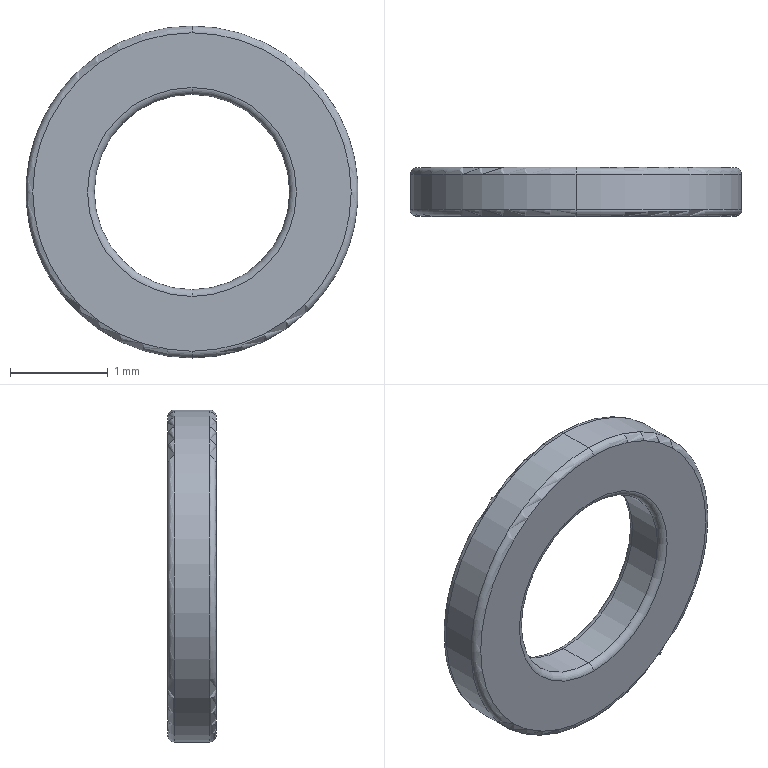Part | SolidWorks | features Extrusion 1, Fillet 1 | 1 solid | 14 faces | box 3.4 x 0.5 x 3.4 mm | volume 2.933 mm3 | torus 8 | cylinder 4 | plane 2 | commonest cylinder face diameters 2 x2 3.4 x2
STEP:
#1=CARTESIAN_POINT('',(0.,0.43,-1.7));
#2=VERTEX_POINT('',#1);
#3=CARTESIAN_POINT('',(0.,0.43,1.7));
#4=VERTEX_POINT('',#3);
#5=CARTESIAN_POINT('',(0.,0.43,0.));
#6=DIRECTION('',(0.,-1.,0.));
#7=DIRECTION('',(0.,0.,1.));
#8=AXIS2_PLACEMENT_3D('',#5,#6,#7);
#9=CIRCLE('',#8,1.7);
#10=EDGE_CURVE('',#2,#4,#9,.T.);
#11=ORIENTED_EDGE('',*,*,#10,.F.);
#12=CARTESIAN_POINT('',(0.,0.5,-1.63));
#13=VERTEX_POINT('',#12);
#14=CARTESIAN_POINT('',(0.,0.43,-1.63));
#15=DIRECTION('',(1.,0.,0.));
#16=DIRECTION('',(0.,0.,-1.));
#17=AXIS2_PLACEMENT_3D('',#14,#15,#16);
#18=CIRCLE('',#17,0.07);
#19=EDGE_CURVE('',#2,#13,#18,.T.);
#20=ORIENTED_EDGE('',*,*,#19,.T.);
#21=CARTESIAN_POINT('',(0.,0.5,1.63));
#22=VERTEX_POINT('',#21);
#23=CARTESIAN_POINT('',(0.,0.5,0.));
#24=DIRECTION('',(0.,1.,0.));
#25=DIRECTION('',(0.,0.,1.));
#26=AXIS2_PLACEMENT_3D('',#23,#24,#25);
#27=CIRCLE('',#26,1.63);
#28=EDGE_CURVE('',#22,#13,#27,.T.);
#29=ORIENTED_EDGE('',*,*,#28,.F.);
#30=CARTESIAN_POINT('',(0.,0.43,1.63));
#31=DIRECTION('',(-1.,0.,0.));
#32=DIRECTION('',(0.,0.,1.));
#33=AXIS2_PLACEMENT_3D('',#30,#31,#32);
#34=CIRCLE('',#33,0.07);
#35=EDGE_CURVE('',#4,#22,#34,.T.);
#36=ORIENTED_EDGE('',*,*,#35,.F.);
#37=EDGE_LOOP('',(#11,#20,#29,#36));
#38=FACE_OUTER_BOUND('',#37,.T.);
#39=CARTESIAN_POINT('',(0.,0.43,0.));
#40=DIRECTION('',(0.,1.,0.));
#41=DIRECTION('',(0.,0.,1.));
#42=AXIS2_PLACEMENT_3D('',#39,#40,#41);
#43=TOROIDAL_SURFACE('',#42,1.63,0.07);
#44=ADVANCED_FACE('',(#38),#43,.T.);
#45=CARTESIAN_POINT('',(0.,0.,-1.63));
#46=VERTEX_POINT('',#45);
#47=CARTESIAN_POINT('',(0.,0.,1.63));
#48=VERTEX_POINT('',#47);
#49=CARTESIAN_POINT('',(0.,0.,0.));
#50=DIRECTION('',(0.,-1.,0.));
#51=DIRECTION('',(0.,0.,1.));
#52=AXIS2_PLACEMENT_3D('',#49,#50,#51);
#53=CIRCLE('',#52,1.63);
#54=EDGE_CURVE('',#46,#48,#53,.T.);
#55=ORIENTED_EDGE('',*,*,#54,.F.);
#56=CARTESIAN_POINT('',(0.,0.07,-1.7));
#57=VERTEX_POINT('',#56);
#58=CARTESIAN_POINT('',(0.,0.07,-1.63));
#59=DIRECTION('',(1.,0.,0.));
#60=DIRECTION('',(0.,0.,-1.));
#61=AXIS2_PLACEMENT_3D('',#58,#59,#60);
#62=CIRCLE('',#61,0.07);
#63=EDGE_CURVE('',#46,#57,#62,.T.);
#64=ORIENTED_EDGE('',*,*,#63,.T.);
#65=CARTESIAN_POINT('',(0.,0.07,1.7));
#66=VERTEX_POINT('',#65);
#67=CARTESIAN_POINT('',(0.,0.07,0.));
#68=DIRECTION('',(0.,1.,0.));
#69=DIRECTION('',(0.,0.,1.));
#70=AXIS2_PLACEMENT_3D('',#67,#68,#69);
#71=CIRCLE('',#70,1.7);
#72=EDGE_CURVE('',#66,#57,#71,.T.);
#73=ORIENTED_EDGE('',*,*,#72,.F.);
#74=CARTESIAN_POINT('',(0.,0.07,1.63));
#75=DIRECTION('',(-1.,0.,0.));
#76=DIRECTION('',(0.,0.,1.));
#77=AXIS2_PLACEMENT_3D('',#74,#75,#76);
#78=CIRCLE('',#77,0.07);
#79=EDGE_CURVE('',#48,#66,#78,.T.);
#80=ORIENTED_EDGE('',*,*,#79,.F.);
#81=EDGE_LOOP('',(#55,#64,#73,#80));
#82=FACE_OUTER_BOUND('',#81,.T.);
#83=CARTESIAN_POINT('',(0.,0.07,0.));
#84=DIRECTION('',(0.,1.,0.));
#85=DIRECTION('',(0.,0.,1.));
#86=AXIS2_PLACEMENT_3D('',#83,#84,#85);
#87=TOROIDAL_SURFACE('',#86,1.63,0.07);
#88=ADVANCED_FACE('',(#82),#87,.T.);
#89=CARTESIAN_POINT('',(0.,0.5,-1.07));
#90=VERTEX_POINT('',#89);
#91=CARTESIAN_POINT('',(0.,0.5,1.07));
#92=VERTEX_POINT('',#91);
#93=CARTESIAN_POINT('',(0.,0.5,0.));
#94=DIRECTION('',(0.,-1.,0.));
#95=DIRECTION('',(0.,0.,1.));
#96=AXIS2_PLACEMENT_3D('',#93,#94,#95);
#97=CIRCLE('',#96,1.07);
#98=EDGE_CURVE('',#90,#92,#97,.T.);
#99=ORIENTED_EDGE('',*,*,#98,.F.);
#100=CARTESIAN_POINT('',(0.,0.43,-1.));
#101=VERTEX_POINT('',#100);
#102=CARTESIAN_POINT('',(0.,0.43,-1.07));
#103=DIRECTION('',(1.,0.,0.));
#104=DIRECTION('',(0.,0.,-1.));
#105=AXIS2_PLACEMENT_3D('',#102,#103,#104);
#106=CIRCLE('',#105,0.07);
#107=EDGE_CURVE('',#90,#101,#106,.T.);
#108=ORIENTED_EDGE('',*,*,#107,.T.);
#109=CARTESIAN_POINT('',(0.,0.43,1.));
#110=VERTEX_POINT('',#109);
#111=CARTESIAN_POINT('',(0.,0.43,0.));
#112=DIRECTION('',(0.,1.,0.));
#113=DIRECTION('',(0.,0.,1.));
#114=AXIS2_PLACEMENT_3D('',#111,#112,#113);
#115=CIRCLE('',#114,1.);
#116=EDGE_CURVE('',#110,#101,#115,.T.);
#117=ORIENTED_EDGE('',*,*,#116,.F.);
#118=CARTESIAN_POINT('',(0.,0.43,1.07));
#119=DIRECTION('',(-1.,0.,0.));
#120=DIRECTION('',(0.,0.,1.));
#121=AXIS2_PLACEMENT_3D('',#118,#119,#120);
#122=CIRCLE('',#121,0.07);
#123=EDGE_CURVE('',#92,#110,#122,.T.);
#124=ORIENTED_EDGE('',*,*,#123,.F.);
#125=EDGE_LOOP('',(#99,#108,#117,#124));
#126=FACE_OUTER_BOUND('',#125,.T.);
#127=CARTESIAN_POINT('',(0.,0.43,0.));
#128=DIRECTION('',(0.,1.,0.));
#129=DIRECTION('',(0.,0.,1.));
#130=AXIS2_PLACEMENT_3D('',#127,#128,#129);
#131=TOROIDAL_SURFACE('',#130,1.07,0.07);
#132=ADVANCED_FACE('',(#126),#131,.T.);
#133=CARTESIAN_POINT('',(0.,0.07,-1.));
#134=VERTEX_POINT('',#133);
#135=CARTESIAN_POINT('',(0.,0.07,1.));
#136=VERTEX_POINT('',#135);
#137=CARTESIAN_POINT('',(0.,0.07,0.));
#138=DIRECTION('',(0.,-1.,0.));
#139=DIRECTION('',(0.,0.,1.));
#140=AXIS2_PLACEMENT_3D('',#137,#138,#139);
#141=CIRCLE('',#140,1.);
#142=EDGE_CURVE('',#134,#136,#141,.T.);
#143=ORIENTED_EDGE('',*,*,#142,.F.);
#144=CARTESIAN_POINT('',(0.,0.,-1.07));
#145=VERTEX_POINT('',#144);
#146=CARTESIAN_POINT('',(0.,0.07,-1.07));
#147=DIRECTION('',(1.,0.,0.));
#148=DIRECTION('',(0.,0.,-1.));
#149=AXIS2_PLACEMENT_3D('',#146,#147,#148);
#150=CIRCLE('',#149,0.07);
#151=EDGE_CURVE('',#134,#145,#150,.T.);
#152=ORIENTED_EDGE('',*,*,#151,.T.);
#153=CARTESIAN_POINT('',(0.,0.,1.07));
#154=VERTEX_POINT('',#153);
#155=CARTESIAN_POINT('',(0.,0.,0.));
#156=DIRECTION('',(0.,1.,0.));
#157=DIRECTION('',(0.,0.,1.));
#158=AXIS2_PLACEMENT_3D('',#155,#156,#157);
#159=CIRCLE('',#158,1.07);
#160=EDGE_CURVE('',#154,#145,#159,.T.);
#161=ORIENTED_EDGE('',*,*,#160,.F.);
#162=CARTESIAN_POINT('',(0.,0.07,1.07));
#163=DIRECTION('',(-1.,0.,0.));
#164=DIRECTION('',(0.,0.,1.));
#165=AXIS2_PLACEMENT_3D('',#162,#163,#164);
#166=CIRCLE('',#165,0.07);
#167=EDGE_CURVE('',#136,#154,#166,.T.);
#168=ORIENTED_EDGE('',*,*,#167,.F.);
#169=EDGE_LOOP('',(#143,#152,#161,#168));
#170=FACE_OUTER_BOUND('',#169,.T.);
#171=CARTESIAN_POINT('',(0.,0.07,0.));
#172=DIRECTION('',(0.,1.,0.));
#173=DIRECTION('',(0.,0.,1.));
#174=AXIS2_PLACEMENT_3D('',#171,#172,#173);
#175=TOROIDAL_SURFACE('',#174,1.07,0.07);
#176=ADVANCED_FACE('',(#170),#175,.T.);
#177=CARTESIAN_POINT('',(0.,0.43,0.));
#178=DIRECTION('',(0.,1.,0.));
#179=DIRECTION('',(0.,0.,1.));
#180=AXIS2_PLACEMENT_3D('',#177,#178,#179);
#181=CIRCLE('',#180,1.);
#182=EDGE_CURVE('',#101,#110,#181,.T.);
#183=ORIENTED_EDGE('',*,*,#182,.T.);
#184=CARTESIAN_POINT('',(0.,0.5,1.));
#185=DIRECTION('',(0.,-1.,0.));
#186=VECTOR('',#185,1000.);
#187=LINE('',#184,#186);
#188=EDGE_CURVE('',#110,#136,#187,.T.);
#189=ORIENTED_EDGE('',*,*,#188,.T.);
#190=CARTESIAN_POINT('',(0.,0.07,0.));
#191=DIRECTION('',(0.,-1.,0.));
#192=DIRECTION('',(0.,0.,1.));
#193=AXIS2_PLACEMENT_3D('',#190,#191,#192);
#194=CIRCLE('',#193,1.);
#195=EDGE_CURVE('',#136,#134,#194,.T.);
#196=ORIENTED_EDGE('',*,*,#195,.T.);
#197=CARTESIAN_POINT('',(0.,0.5,-1.));
#198=DIRECTION('',(0.,-1.,0.));
#199=VECTOR('',#198,1000.);
#200=LINE('',#197,#199);
#201=EDGE_CURVE('',#101,#134,#200,.T.);
#202=ORIENTED_EDGE('',*,*,#201,.F.);
#203=EDGE_LOOP('',(#183,#189,#196,#202));
#204=FACE_OUTER_BOUND('',#203,.T.);
#205=CARTESIAN_POINT('',(0.,0.5,0.));
#206=DIRECTION('',(0.,-1.,0.));
#207=DIRECTION('',(0.,0.,-1.));
#208=AXIS2_PLACEMENT_3D('',#205,#206,#207);
#209=CYLINDRICAL_SURFACE('',#208,1.);
#210=ADVANCED_FACE('',(#204),#209,.F.);
#211=ORIENTED_EDGE('',*,*,#10,.T.);
#212=CARTESIAN_POINT('',(0.,0.5,1.7));
#213=DIRECTION('',(0.,-1.,0.));
#214=VECTOR('',#213,1000.);
#215=LINE('',#212,#214);
#216=EDGE_CURVE('',#4,#66,#215,.T.);
#217=ORIENTED_EDGE('',*,*,#216,.T.);
#218=ORIENTED_EDGE('',*,*,#72,.T.);
#219=CARTESIAN_POINT('',(0.,0.5,-1.7));
#220=DIRECTION('',(0.,-1.,0.));
#221=VECTOR('',#220,1000.);
#222=LINE('',#219,#221);
#223=EDGE_CURVE('',#2,#57,#222,.T.);
#224=ORIENTED_EDGE('',*,*,#223,.F.);
#225=EDGE_LOOP('',(#211,#217,#218,#224));
#226=FACE_OUTER_BOUND('',#225,.T.);
#227=CARTESIAN_POINT('',(0.,0.5,0.));
#228=DIRECTION('',(0.,-1.,0.));
#229=DIRECTION('',(0.,0.,-1.));
#230=AXIS2_PLACEMENT_3D('',#227,#228,#229);
#231=CYLINDRICAL_SURFACE('',#230,1.7);
#232=ADVANCED_FACE('',(#226),#231,.T.);
#233=CARTESIAN_POINT('',(0.,0.5,0.));
#234=DIRECTION('',(0.,-1.,0.));
#235=DIRECTION('',(0.,0.,1.));
#236=AXIS2_PLACEMENT_3D('',#233,#234,#235);
#237=CIRCLE('',#236,1.07);
#238=EDGE_CURVE('',#92,#90,#237,.T.);
#239=ORIENTED_EDGE('',*,*,#238,.T.);
#240=ORIENTED_EDGE('',*,*,#98,.T.);
#241=EDGE_LOOP('',(#239,#240));
#242=FACE_BOUND('',#241,.T.);
#243=ORIENTED_EDGE('',*,*,#28,.T.);
#244=CARTESIAN_POINT('',(0.,0.5,0.));
#245=DIRECTION('',(0.,1.,0.));
#246=DIRECTION('',(0.,0.,1.));
#247=AXIS2_PLACEMENT_3D('',#244,#245,#246);
#248=CIRCLE('',#247,1.63);
#249=EDGE_CURVE('',#13,#22,#248,.T.);
#250=ORIENTED_EDGE('',*,*,#249,.T.);
#251=EDGE_LOOP('',(#243,#250));
#252=FACE_OUTER_BOUND('',#251,.T.);
#253=CARTESIAN_POINT('',(0.,0.5,0.));
#254=DIRECTION('',(0.,1.,0.));
#255=DIRECTION('',(0.,0.,1.));
#256=AXIS2_PLACEMENT_3D('',#253,#254,#255);
#257=PLANE('',#256);
#258=ADVANCED_FACE('',(#242,#252),#257,.T.);
#259=ORIENTED_EDGE('',*,*,#160,.T.);
#260=CARTESIAN_POINT('',(0.,0.,0.));
#261=DIRECTION('',(0.,1.,0.));
#262=DIRECTION('',(0.,0.,1.));
#263=AXIS2_PLACEMENT_3D('',#260,#261,#262);
#264=CIRCLE('',#263,1.07);
#265=EDGE_CURVE('',#145,#154,#264,.T.);
#266=ORIENTED_EDGE('',*,*,#265,.T.);
#267=EDGE_LOOP('',(#259,#266));
#268=FACE_BOUND('',#267,.T.);
#269=CARTESIAN_POINT('',(0.,0.,0.));
#270=DIRECTION('',(0.,-1.,0.));
#271=DIRECTION('',(0.,0.,1.));
#272=AXIS2_PLACEMENT_3D('',#269,#270,#271);
#273=CIRCLE('',#272,1.63);
#274=EDGE_CURVE('',#48,#46,#273,.T.);
#275=ORIENTED_EDGE('',*,*,#274,.T.);
#276=ORIENTED_EDGE('',*,*,#54,.T.);
#277=EDGE_LOOP('',(#275,#276));
#278=FACE_OUTER_BOUND('',#277,.T.);
#279=CARTESIAN_POINT('',(0.,0.,0.));
#280=DIRECTION('',(0.,1.,0.));
#281=DIRECTION('',(0.,0.,1.));
#282=AXIS2_PLACEMENT_3D('',#279,#280,#281);
#283=PLANE('',#282);
#284=ADVANCED_FACE('',(#268,#278),#283,.F.);
#285=ORIENTED_EDGE('',*,*,#216,.F.);
#286=CARTESIAN_POINT('',(0.,0.43,0.));
#287=DIRECTION('',(0.,-1.,0.));
#288=DIRECTION('',(0.,0.,1.));
#289=AXIS2_PLACEMENT_3D('',#286,#287,#288);
#290=CIRCLE('',#289,1.7);
#291=EDGE_CURVE('',#4,#2,#290,.T.);
#292=ORIENTED_EDGE('',*,*,#291,.T.);
#293=ORIENTED_EDGE('',*,*,#223,.T.);
#294=CARTESIAN_POINT('',(0.,0.07,0.));
#295=DIRECTION('',(0.,1.,0.));
#296=DIRECTION('',(0.,0.,1.));
#297=AXIS2_PLACEMENT_3D('',#294,#295,#296);
#298=CIRCLE('',#297,1.7);
#299=EDGE_CURVE('',#57,#66,#298,.T.);
#300=ORIENTED_EDGE('',*,*,#299,.T.);
#301=EDGE_LOOP('',(#285,#292,#293,#300));
#302=FACE_OUTER_BOUND('',#301,.T.);
#303=CARTESIAN_POINT('',(0.,0.5,0.));
#304=DIRECTION('',(0.,-1.,0.));
#305=DIRECTION('',(0.,0.,-1.));
#306=AXIS2_PLACEMENT_3D('',#303,#304,#305);
#307=CYLINDRICAL_SURFACE('',#306,1.7);
#308=ADVANCED_FACE('',(#302),#307,.T.);
#309=ORIENTED_EDGE('',*,*,#188,.F.);
#310=ORIENTED_EDGE('',*,*,#116,.T.);
#311=ORIENTED_EDGE('',*,*,#201,.T.);
#312=ORIENTED_EDGE('',*,*,#142,.T.);
#313=EDGE_LOOP('',(#309,#310,#311,#312));
#314=FACE_OUTER_BOUND('',#313,.T.);
#315=CARTESIAN_POINT('',(0.,0.5,0.));
#316=DIRECTION('',(0.,-1.,0.));
#317=DIRECTION('',(0.,0.,-1.));
#318=AXIS2_PLACEMENT_3D('',#315,#316,#317);
#319=CYLINDRICAL_SURFACE('',#318,1.);
#320=ADVANCED_FACE('',(#314),#319,.F.);
#321=ORIENTED_EDGE('',*,*,#151,.F.);
#322=ORIENTED_EDGE('',*,*,#195,.F.);
#323=ORIENTED_EDGE('',*,*,#167,.T.);
#324=ORIENTED_EDGE('',*,*,#265,.F.);
#325=EDGE_LOOP('',(#321,#322,#323,#324));
#326=FACE_OUTER_BOUND('',#325,.T.);
#327=CARTESIAN_POINT('',(0.,0.07,0.));
#328=DIRECTION('',(0.,1.,0.));
#329=DIRECTION('',(0.,0.,1.));
#330=AXIS2_PLACEMENT_3D('',#327,#328,#329);
#331=TOROIDAL_SURFACE('',#330,1.07,0.07);
#332=ADVANCED_FACE('',(#326),#331,.T.);
#333=ORIENTED_EDGE('',*,*,#107,.F.);
#334=ORIENTED_EDGE('',*,*,#238,.F.);
#335=ORIENTED_EDGE('',*,*,#123,.T.);
#336=ORIENTED_EDGE('',*,*,#182,.F.);
#337=EDGE_LOOP('',(#333,#334,#335,#336));
#338=FACE_OUTER_BOUND('',#337,.T.);
#339=CARTESIAN_POINT('',(0.,0.43,0.));
#340=DIRECTION('',(0.,1.,0.));
#341=DIRECTION('',(0.,0.,1.));
#342=AXIS2_PLACEMENT_3D('',#339,#340,#341);
#343=TOROIDAL_SURFACE('',#342,1.07,0.07);
#344=ADVANCED_FACE('',(#338),#343,.T.);
#345=ORIENTED_EDGE('',*,*,#63,.F.);
#346=ORIENTED_EDGE('',*,*,#274,.F.);
#347=ORIENTED_EDGE('',*,*,#79,.T.);
#348=ORIENTED_EDGE('',*,*,#299,.F.);
#349=EDGE_LOOP('',(#345,#346,#347,#348));
#350=FACE_OUTER_BOUND('',#349,.T.);
#351=CARTESIAN_POINT('',(0.,0.07,0.));
#352=DIRECTION('',(0.,1.,0.));
#353=DIRECTION('',(0.,0.,1.));
#354=AXIS2_PLACEMENT_3D('',#351,#352,#353);
#355=TOROIDAL_SURFACE('',#354,1.63,0.07);
#356=ADVANCED_FACE('',(#350),#355,.T.);
#357=ORIENTED_EDGE('',*,*,#19,.F.);
#358=ORIENTED_EDGE('',*,*,#291,.F.);
#359=ORIENTED_EDGE('',*,*,#35,.T.);
#360=ORIENTED_EDGE('',*,*,#249,.F.);
#361=EDGE_LOOP('',(#357,#358,#359,#360));
#362=FACE_OUTER_BOUND('',#361,.T.);
#363=CARTESIAN_POINT('',(0.,0.43,0.));
#364=DIRECTION('',(0.,1.,0.));
#365=DIRECTION('',(0.,0.,1.));
#366=AXIS2_PLACEMENT_3D('',#363,#364,#365);
#367=TOROIDAL_SURFACE('',#366,1.63,0.07);
#368=ADVANCED_FACE('',(#362),#367,.T.);
#369=CLOSED_SHELL('',(#44,#88,#132,#176,#210,#232,#258,#284,#308,#320,#332,#344,#356,#368));
#370=MANIFOLD_SOLID_BREP('',#369);
#371=CARTESIAN_POINT('',(0.,0.,0.));
#372=DIRECTION('',(0.,0.,1.));
#373=DIRECTION('',(1.,0.,0.));
#374=AXIS2_PLACEMENT_3D('',#371,#372,#373);
#375=(LENGTH_UNIT()NAMED_UNIT(*)SI_UNIT(.MILLI.,.METRE.));
#376=UNCERTAINTY_MEASURE_WITH_UNIT(LENGTH_MEASURE(0.00001),#375,'','');
#377=(NAMED_UNIT(*)PLANE_ANGLE_UNIT()SI_UNIT($,.RADIAN.));
#378=(NAMED_UNIT(*)SI_UNIT($,.STERADIAN.)SOLID_ANGLE_UNIT());
#379=(GEOMETRIC_REPRESENTATION_CONTEXT(3)GLOBAL_UNCERTAINTY_ASSIGNED_CONTEXT((#376))GLOBAL_UNIT_ASSIGNED_CONTEXT((#375,#377,#378))REPRESENTATION_CONTEXT('',''));
#380=ADVANCED_BREP_SHAPE_REPRESENTATION('',(#370,#374),#379);